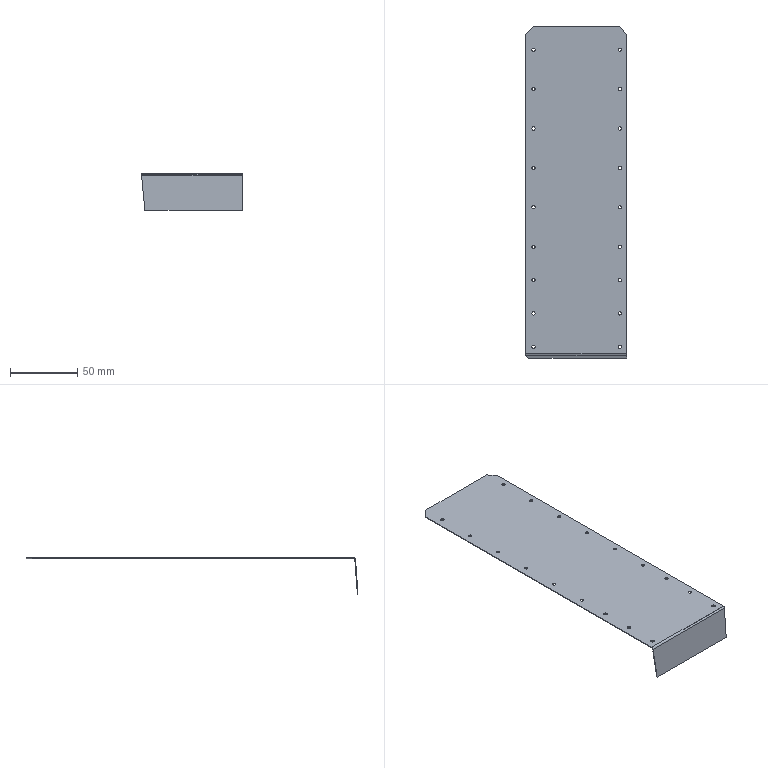Part | SolidWorks | features BaseBody 1 | 1 solid | 52 faces | box 74.9 x 245.929 x 26.779 mm | volume 10028 mm3 | cylinder 38 | plane 12 | spline 2 | commonest cylinder face diameters 2.4 x36 1.473 x1 2.473 x1